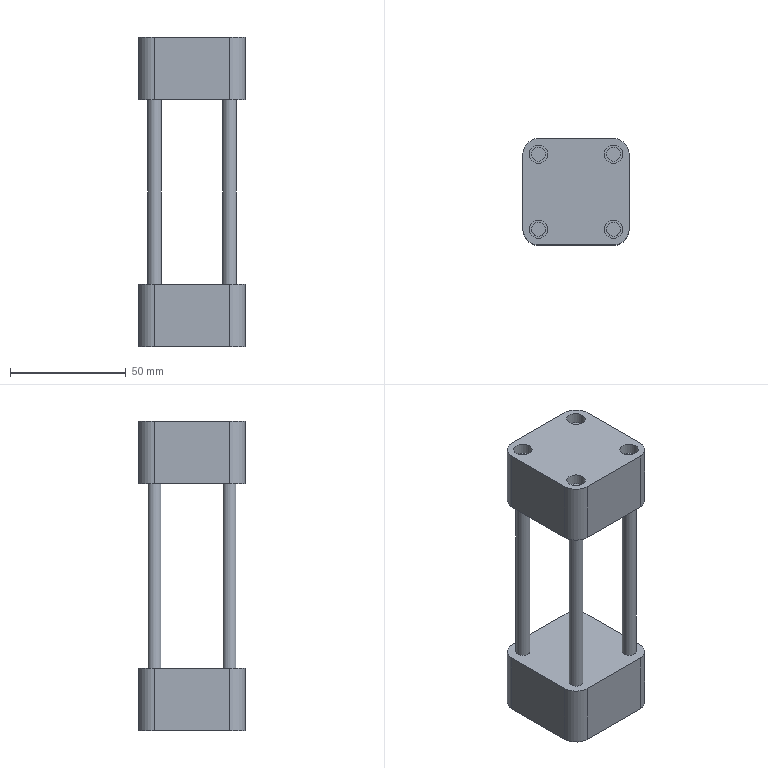Part | NX | features solid 2 | 1 solid | 48 faces | box 46 x 46 x 134 mm | volume 118030 mm3 | plane 24 | cylinder 24 | commonest cylinder face diameters 6 x8 13.5 x8 8 x4 6.667 x2 10 x2
STEP:
#1=CARTESIAN_POINT('',(312.,-98.75,-137.));
#2=VERTEX_POINT('',#1);
#3=CARTESIAN_POINT('',(312.,-131.25,-137.));
#4=VERTEX_POINT('',#3);
#5=CARTESIAN_POINT('',(312.,-92.,-137.));
#6=DIRECTION('',(0.,-1.,0.));
#7=VECTOR('',#6,1000.);
#8=LINE('',#5,#7);
#9=EDGE_CURVE('',#2,#4,#8,.T.);
#10=ORIENTED_EDGE('',*,*,#9,.F.);
#11=CARTESIAN_POINT('',(312.,-98.75,-164.));
#12=VERTEX_POINT('',#11);
#13=CARTESIAN_POINT('',(312.,-98.75,-164.));
#14=DIRECTION('',(0.,0.,-1.));
#15=VECTOR('',#14,1000.);
#16=LINE('',#13,#15);
#17=EDGE_CURVE('',#2,#12,#16,.T.);
#18=ORIENTED_EDGE('',*,*,#17,.T.);
#19=CARTESIAN_POINT('',(312.,-131.25,-164.));
#20=VERTEX_POINT('',#19);
#21=CARTESIAN_POINT('',(312.,-92.,-164.));
#22=DIRECTION('',(0.,-1.,0.));
#23=VECTOR('',#22,1000.);
#24=LINE('',#21,#23);
#25=EDGE_CURVE('',#12,#20,#24,.T.);
#26=ORIENTED_EDGE('',*,*,#25,.T.);
#27=CARTESIAN_POINT('',(312.,-131.25,-137.));
#28=DIRECTION('',(0.,0.,-1.));
#29=VECTOR('',#28,1000.);
#30=LINE('',#27,#29);
#31=EDGE_CURVE('',#20,#4,#30,.F.);
#32=ORIENTED_EDGE('',*,*,#31,.T.);
#33=EDGE_LOOP('',(#10,#18,#26,#32));
#34=FACE_BOUND('',#33,.T.);
#35=CARTESIAN_POINT('',(312.,-92.,-137.));
#36=DIRECTION('',(1.,0.,0.));
#37=DIRECTION('',(0.,1.,0.));
#38=AXIS2_PLACEMENT_3D('',#35,#36,#37);
#39=PLANE('',#38);
#40=ADVANCED_FACE('',(#34),#39,.F.);
#41=CARTESIAN_POINT('',(351.25,-138.,-137.));
#42=VERTEX_POINT('',#41);
#43=CARTESIAN_POINT('',(318.75,-138.,-137.));
#44=VERTEX_POINT('',#43);
#45=CARTESIAN_POINT('',(358.,-138.,-137.));
#46=DIRECTION('',(-1.,0.,0.));
#47=VECTOR('',#46,1000.);
#48=LINE('',#45,#47);
#49=EDGE_CURVE('',#42,#44,#48,.T.);
#50=ORIENTED_EDGE('',*,*,#49,.T.);
#51=CARTESIAN_POINT('',(318.75,-138.,-164.));
#52=VERTEX_POINT('',#51);
#53=CARTESIAN_POINT('',(318.75,-138.,-164.));
#54=DIRECTION('',(0.,0.,-1.));
#55=VECTOR('',#54,1000.);
#56=LINE('',#53,#55);
#57=EDGE_CURVE('',#44,#52,#56,.T.);
#58=ORIENTED_EDGE('',*,*,#57,.T.);
#59=CARTESIAN_POINT('',(351.25,-138.,-164.));
#60=VERTEX_POINT('',#59);
#61=CARTESIAN_POINT('',(358.,-138.,-164.));
#62=DIRECTION('',(-1.,0.,0.));
#63=VECTOR('',#62,1000.);
#64=LINE('',#61,#63);
#65=EDGE_CURVE('',#60,#52,#64,.T.);
#66=ORIENTED_EDGE('',*,*,#65,.F.);
#67=CARTESIAN_POINT('',(351.25,-138.,-137.));
#68=DIRECTION('',(0.,0.,-1.));
#69=VECTOR('',#68,1000.);
#70=LINE('',#67,#69);
#71=EDGE_CURVE('',#60,#42,#70,.F.);
#72=ORIENTED_EDGE('',*,*,#71,.T.);
#73=EDGE_LOOP('',(#50,#58,#66,#72));
#74=FACE_BOUND('',#73,.T.);
#75=CARTESIAN_POINT('',(358.,-138.,-137.));
#76=DIRECTION('',(0.,-1.,0.));
#77=DIRECTION('',(1.,0.,0.));
#78=AXIS2_PLACEMENT_3D('',#75,#76,#77);
#79=PLANE('',#78);
#80=ADVANCED_FACE('',(#74),#79,.T.);
#81=CARTESIAN_POINT('',(358.,-131.25,-164.));
#82=VERTEX_POINT('',#81);
#83=CARTESIAN_POINT('',(358.,-98.75,-164.));
#84=VERTEX_POINT('',#83);
#85=CARTESIAN_POINT('',(358.,-138.,-164.));
#86=DIRECTION('',(0.,1.,0.));
#87=VECTOR('',#86,1000.);
#88=LINE('',#85,#87);
#89=EDGE_CURVE('',#82,#84,#88,.T.);
#90=ORIENTED_EDGE('',*,*,#89,.T.);
#91=CARTESIAN_POINT('',(358.,-98.75,-137.));
#92=VERTEX_POINT('',#91);
#93=CARTESIAN_POINT('',(358.,-98.75,-137.));
#94=DIRECTION('',(0.,0.,-1.));
#95=VECTOR('',#94,1000.);
#96=LINE('',#93,#95);
#97=EDGE_CURVE('',#84,#92,#96,.F.);
#98=ORIENTED_EDGE('',*,*,#97,.T.);
#99=CARTESIAN_POINT('',(358.,-131.25,-137.));
#100=VERTEX_POINT('',#99);
#101=CARTESIAN_POINT('',(358.,-138.,-137.));
#102=DIRECTION('',(0.,1.,0.));
#103=VECTOR('',#102,1000.);
#104=LINE('',#101,#103);
#105=EDGE_CURVE('',#100,#92,#104,.T.);
#106=ORIENTED_EDGE('',*,*,#105,.F.);
#107=CARTESIAN_POINT('',(358.,-131.25,-164.));
#108=DIRECTION('',(0.,0.,-1.));
#109=VECTOR('',#108,1000.);
#110=LINE('',#107,#109);
#111=EDGE_CURVE('',#100,#82,#110,.T.);
#112=ORIENTED_EDGE('',*,*,#111,.T.);
#113=EDGE_LOOP('',(#90,#98,#106,#112));
#114=FACE_BOUND('',#113,.T.);
#115=CARTESIAN_POINT('',(358.,-138.,-137.));
#116=DIRECTION('',(-1.,0.,0.));
#117=DIRECTION('',(0.,-1.,0.));
#118=AXIS2_PLACEMENT_3D('',#115,#116,#117);
#119=PLANE('',#118);
#120=ADVANCED_FACE('',(#114),#119,.F.);
#121=CARTESIAN_POINT('',(341.5,-92.,-151.833));
#122=VERTEX_POINT('',#121);
#123=CARTESIAN_POINT('',(341.5,-92.,-148.5));
#124=DIRECTION('',(0.,-1.,0.));
#125=DIRECTION('',(0.,0.,-1.));
#126=AXIS2_PLACEMENT_3D('',#123,#124,#125);
#127=CIRCLE('',#126,3.333);
#128=EDGE_CURVE('',#122,#122,#127,.T.);
#129=ORIENTED_EDGE('',*,*,#128,.T.);
#130=EDGE_LOOP('',(#129));
#131=FACE_BOUND('',#130,.T.);
#132=CARTESIAN_POINT('',(331.,-92.,-156.));
#133=VERTEX_POINT('',#132);
#134=CARTESIAN_POINT('',(331.,-92.,-151.));
#135=DIRECTION('',(0.,-1.,0.));
#136=DIRECTION('',(0.,0.,-1.));
#137=AXIS2_PLACEMENT_3D('',#134,#135,#136);
#138=CIRCLE('',#137,5.);
#139=EDGE_CURVE('',#133,#133,#138,.T.);
#140=ORIENTED_EDGE('',*,*,#139,.T.);
#141=EDGE_LOOP('',(#140));
#142=FACE_BOUND('',#141,.T.);
#143=CARTESIAN_POINT('',(318.75,-92.,-164.));
#144=VERTEX_POINT('',#143);
#145=CARTESIAN_POINT('',(351.25,-92.,-164.));
#146=VERTEX_POINT('',#145);
#147=CARTESIAN_POINT('',(312.,-92.,-164.));
#148=DIRECTION('',(1.,0.,0.));
#149=VECTOR('',#148,1000.);
#150=LINE('',#147,#149);
#151=EDGE_CURVE('',#144,#146,#150,.T.);
#152=ORIENTED_EDGE('',*,*,#151,.F.);
#153=CARTESIAN_POINT('',(318.75,-92.,-137.));
#154=VERTEX_POINT('',#153);
#155=CARTESIAN_POINT('',(318.75,-92.,-137.));
#156=DIRECTION('',(0.,0.,-1.));
#157=VECTOR('',#156,1000.);
#158=LINE('',#155,#157);
#159=EDGE_CURVE('',#144,#154,#158,.F.);
#160=ORIENTED_EDGE('',*,*,#159,.T.);
#161=CARTESIAN_POINT('',(351.25,-92.,-137.));
#162=VERTEX_POINT('',#161);
#163=CARTESIAN_POINT('',(312.,-92.,-137.));
#164=DIRECTION('',(1.,0.,0.));
#165=VECTOR('',#164,1000.);
#166=LINE('',#163,#165);
#167=EDGE_CURVE('',#154,#162,#166,.T.);
#168=ORIENTED_EDGE('',*,*,#167,.T.);
#169=CARTESIAN_POINT('',(351.25,-92.,-164.));
#170=DIRECTION('',(0.,0.,-1.));
#171=VECTOR('',#170,1000.);
#172=LINE('',#169,#171);
#173=EDGE_CURVE('',#162,#146,#172,.T.);
#174=ORIENTED_EDGE('',*,*,#173,.T.);
#175=EDGE_LOOP('',(#152,#160,#168,#174));
#176=FACE_BOUND('',#175,.T.);
#177=CARTESIAN_POINT('',(312.,-92.,-137.));
#178=DIRECTION('',(0.,1.,0.));
#179=DIRECTION('',(0.,0.,1.));
#180=AXIS2_PLACEMENT_3D('',#177,#178,#179);
#181=PLANE('',#180);
#182=ADVANCED_FACE('',(#131,#142,#176),#181,.T.);
#183=CARTESIAN_POINT('',(348.25,-98.75,-137.));
#184=VERTEX_POINT('',#183);
#185=CARTESIAN_POINT('',(351.25,-98.75,-137.));
#186=DIRECTION('',(0.,0.,1.));
#187=DIRECTION('',(-1.,0.,0.));
#188=AXIS2_PLACEMENT_3D('',#185,#186,#187);
#189=CIRCLE('',#188,3.);
#190=EDGE_CURVE('',#184,#184,#189,.T.);
#191=ORIENTED_EDGE('',*,*,#190,.F.);
#192=EDGE_LOOP('',(#191));
#193=FACE_BOUND('',#192,.T.);
#194=CARTESIAN_POINT('',(321.75,-98.75,-137.));
#195=VERTEX_POINT('',#194);
#196=CARTESIAN_POINT('',(318.75,-98.75,-137.));
#197=DIRECTION('',(0.,0.,-1.));
#198=DIRECTION('',(1.,0.,0.));
#199=AXIS2_PLACEMENT_3D('',#196,#197,#198);
#200=CIRCLE('',#199,3.);
#201=EDGE_CURVE('',#195,#195,#200,.T.);
#202=ORIENTED_EDGE('',*,*,#201,.T.);
#203=EDGE_LOOP('',(#202));
#204=FACE_BOUND('',#203,.T.);
#205=CARTESIAN_POINT('',(348.25,-131.25,-137.));
#206=VERTEX_POINT('',#205);
#207=CARTESIAN_POINT('',(351.25,-131.25,-137.));
#208=DIRECTION('',(0.,0.,-1.));
#209=DIRECTION('',(-1.,0.,0.));
#210=AXIS2_PLACEMENT_3D('',#207,#208,#209);
#211=CIRCLE('',#210,3.);
#212=EDGE_CURVE('',#206,#206,#211,.T.);
#213=ORIENTED_EDGE('',*,*,#212,.T.);
#214=EDGE_LOOP('',(#213));
#215=FACE_BOUND('',#214,.T.);
#216=CARTESIAN_POINT('',(321.75,-131.25,-137.));
#217=VERTEX_POINT('',#216);
#218=CARTESIAN_POINT('',(318.75,-131.25,-137.));
#219=DIRECTION('',(0.,0.,1.));
#220=DIRECTION('',(1.,0.,0.));
#221=AXIS2_PLACEMENT_3D('',#218,#219,#220);
#222=CIRCLE('',#221,3.);
#223=EDGE_CURVE('',#217,#217,#222,.T.);
#224=ORIENTED_EDGE('',*,*,#223,.F.);
#225=EDGE_LOOP('',(#224));
#226=FACE_BOUND('',#225,.T.);
#227=ORIENTED_EDGE('',*,*,#167,.F.);
#228=CARTESIAN_POINT('',(318.75,-98.75,-137.));
#229=DIRECTION('',(0.,0.,-1.));
#230=DIRECTION('',(-1.,0.,0.));
#231=AXIS2_PLACEMENT_3D('',#228,#229,#230);
#232=CIRCLE('',#231,6.75);
#233=EDGE_CURVE('',#154,#2,#232,.F.);
#234=ORIENTED_EDGE('',*,*,#233,.T.);
#235=ORIENTED_EDGE('',*,*,#9,.T.);
#236=CARTESIAN_POINT('',(318.75,-131.25,-137.));
#237=DIRECTION('',(0.,0.,-1.));
#238=DIRECTION('',(-1.,0.,0.));
#239=AXIS2_PLACEMENT_3D('',#236,#237,#238);
#240=CIRCLE('',#239,6.75);
#241=EDGE_CURVE('',#4,#44,#240,.F.);
#242=ORIENTED_EDGE('',*,*,#241,.T.);
#243=ORIENTED_EDGE('',*,*,#49,.F.);
#244=CARTESIAN_POINT('',(351.25,-131.25,-137.));
#245=DIRECTION('',(0.,0.,-1.));
#246=DIRECTION('',(-1.,0.,0.));
#247=AXIS2_PLACEMENT_3D('',#244,#245,#246);
#248=CIRCLE('',#247,6.75);
#249=EDGE_CURVE('',#42,#100,#248,.F.);
#250=ORIENTED_EDGE('',*,*,#249,.T.);
#251=ORIENTED_EDGE('',*,*,#105,.T.);
#252=CARTESIAN_POINT('',(351.25,-98.75,-137.));
#253=DIRECTION('',(0.,0.,-1.));
#254=DIRECTION('',(-1.,0.,0.));
#255=AXIS2_PLACEMENT_3D('',#252,#253,#254);
#256=CIRCLE('',#255,6.75);
#257=EDGE_CURVE('',#92,#162,#256,.F.);
#258=ORIENTED_EDGE('',*,*,#257,.T.);
#259=EDGE_LOOP('',(#227,#234,#235,#242,#243,#250,#251,#258));
#260=FACE_BOUND('',#259,.T.);
#261=CARTESIAN_POINT('',(312.,-138.,-137.));
#262=DIRECTION('',(0.,0.,-1.));
#263=DIRECTION('',(-1.,0.,0.));
#264=AXIS2_PLACEMENT_3D('',#261,#262,#263);
#265=PLANE('',#264);
#266=ADVANCED_FACE('',(#193,#204,#215,#226,#260),#265,.F.);
#267=ORIENTED_EDGE('',*,*,#25,.F.);
#268=CARTESIAN_POINT('',(318.75,-98.75,-164.));
#269=DIRECTION('',(0.,0.,-1.));
#270=DIRECTION('',(-1.,0.,0.));
#271=AXIS2_PLACEMENT_3D('',#268,#269,#270);
#272=CIRCLE('',#271,6.75);
#273=EDGE_CURVE('',#12,#144,#272,.T.);
#274=ORIENTED_EDGE('',*,*,#273,.T.);
#275=ORIENTED_EDGE('',*,*,#151,.T.);
#276=CARTESIAN_POINT('',(351.25,-98.75,-164.));
#277=DIRECTION('',(0.,0.,-1.));
#278=DIRECTION('',(-1.,0.,0.));
#279=AXIS2_PLACEMENT_3D('',#276,#277,#278);
#280=CIRCLE('',#279,6.75);
#281=EDGE_CURVE('',#146,#84,#280,.T.);
#282=ORIENTED_EDGE('',*,*,#281,.T.);
#283=ORIENTED_EDGE('',*,*,#89,.F.);
#284=CARTESIAN_POINT('',(351.25,-131.25,-164.));
#285=DIRECTION('',(0.,0.,-1.));
#286=DIRECTION('',(-1.,0.,0.));
#287=AXIS2_PLACEMENT_3D('',#284,#285,#286);
#288=CIRCLE('',#287,6.75);
#289=EDGE_CURVE('',#82,#60,#288,.T.);
#290=ORIENTED_EDGE('',*,*,#289,.T.);
#291=ORIENTED_EDGE('',*,*,#65,.T.);
#292=CARTESIAN_POINT('',(318.75,-131.25,-164.));
#293=DIRECTION('',(0.,0.,-1.));
#294=DIRECTION('',(-1.,0.,0.));
#295=AXIS2_PLACEMENT_3D('',#292,#293,#294);
#296=CIRCLE('',#295,6.75);
#297=EDGE_CURVE('',#52,#20,#296,.T.);
#298=ORIENTED_EDGE('',*,*,#297,.T.);
#299=EDGE_LOOP('',(#267,#274,#275,#282,#283,#290,#291,#298));
#300=FACE_BOUND('',#299,.T.);
#301=CARTESIAN_POINT('',(312.,-138.,-164.));
#302=DIRECTION('',(0.,0.,-1.));
#303=DIRECTION('',(-1.,0.,0.));
#304=AXIS2_PLACEMENT_3D('',#301,#302,#303);
#305=PLANE('',#304);
#306=ADVANCED_FACE('',(#300),#305,.T.);
#307=ORIENTED_EDGE('',*,*,#233,.F.);
#308=ORIENTED_EDGE('',*,*,#159,.F.);
#309=ORIENTED_EDGE('',*,*,#273,.F.);
#310=ORIENTED_EDGE('',*,*,#17,.F.);
#311=EDGE_LOOP('',(#307,#308,#309,#310));
#312=FACE_BOUND('',#311,.T.);
#313=CARTESIAN_POINT('',(318.75,-98.75,-137.));
#314=DIRECTION('',(0.,0.,1.));
#315=DIRECTION('',(1.,0.,0.));
#316=AXIS2_PLACEMENT_3D('',#313,#314,#315);
#317=CYLINDRICAL_SURFACE('',#316,6.75);
#318=ADVANCED_FACE('',(#312),#317,.T.);
#319=ORIENTED_EDGE('',*,*,#241,.F.);
#320=ORIENTED_EDGE('',*,*,#31,.F.);
#321=ORIENTED_EDGE('',*,*,#297,.F.);
#322=ORIENTED_EDGE('',*,*,#57,.F.);
#323=EDGE_LOOP('',(#319,#320,#321,#322));
#324=FACE_BOUND('',#323,.T.);
#325=CARTESIAN_POINT('',(318.75,-131.25,-137.));
#326=DIRECTION('',(0.,0.,1.));
#327=DIRECTION('',(1.,0.,0.));
#328=AXIS2_PLACEMENT_3D('',#325,#326,#327);
#329=CYLINDRICAL_SURFACE('',#328,6.75);
#330=ADVANCED_FACE('',(#324),#329,.T.);
#331=ORIENTED_EDGE('',*,*,#257,.F.);
#332=ORIENTED_EDGE('',*,*,#97,.F.);
#333=ORIENTED_EDGE('',*,*,#281,.F.);
#334=ORIENTED_EDGE('',*,*,#173,.F.);
#335=EDGE_LOOP('',(#331,#332,#333,#334));
#336=FACE_BOUND('',#335,.T.);
#337=CARTESIAN_POINT('',(351.25,-98.75,-137.));
#338=DIRECTION('',(0.,0.,1.));
#339=DIRECTION('',(1.,0.,0.));
#340=AXIS2_PLACEMENT_3D('',#337,#338,#339);
#341=CYLINDRICAL_SURFACE('',#340,6.75);
#342=ADVANCED_FACE('',(#336),#341,.T.);
#343=ORIENTED_EDGE('',*,*,#249,.F.);
#344=ORIENTED_EDGE('',*,*,#71,.F.);
#345=ORIENTED_EDGE('',*,*,#289,.F.);
#346=ORIENTED_EDGE('',*,*,#111,.F.);
#347=EDGE_LOOP('',(#343,#344,#345,#346));
#348=FACE_BOUND('',#347,.T.);
#349=CARTESIAN_POINT('',(351.25,-131.25,-137.));
#350=DIRECTION('',(0.,0.,1.));
#351=DIRECTION('',(1.,0.,0.));
#352=AXIS2_PLACEMENT_3D('',#349,#350,#351);
#353=CYLINDRICAL_SURFACE('',#352,6.75);
#354=ADVANCED_FACE('',(#348),#353,.T.);
#355=CARTESIAN_POINT('',(315.75,-131.25,-57.));
#356=VERTEX_POINT('',#355);
#357=CARTESIAN_POINT('',(318.75,-131.25,-57.));
#358=DIRECTION('',(0.,0.,-1.));
#359=DIRECTION('',(-1.,0.,0.));
#360=AXIS2_PLACEMENT_3D('',#357,#358,#359);
#361=CIRCLE('',#360,3.);
#362=EDGE_CURVE('',#356,#356,#361,.F.);
#363=ORIENTED_EDGE('',*,*,#362,.F.);
#364=EDGE_LOOP('',(#363));
#365=FACE_BOUND('',#364,.T.);
#366=ORIENTED_EDGE('',*,*,#223,.T.);
#367=EDGE_LOOP('',(#366));
#368=FACE_BOUND('',#367,.T.);
#369=CARTESIAN_POINT('',(318.75,-131.25,-137.));
#370=DIRECTION('',(0.,0.,1.));
#371=DIRECTION('',(1.,0.,0.));
#372=AXIS2_PLACEMENT_3D('',#369,#370,#371);
#373=CYLINDRICAL_SURFACE('',#372,3.);
#374=ADVANCED_FACE('',(#365,#368),#373,.T.);
#375=CARTESIAN_POINT('',(348.25,-131.25,-57.));
#376=VERTEX_POINT('',#375);
#377=CARTESIAN_POINT('',(351.25,-131.25,-57.));
#378=DIRECTION('',(0.,0.,-1.));
#379=DIRECTION('',(-1.,0.,0.));
#380=AXIS2_PLACEMENT_3D('',#377,#378,#379);
#381=CIRCLE('',#380,3.);
#382=EDGE_CURVE('',#376,#376,#381,.F.);
#383=ORIENTED_EDGE('',*,*,#382,.F.);
#384=EDGE_LOOP('',(#383));
#385=FACE_BOUND('',#384,.T.);
#386=ORIENTED_EDGE('',*,*,#212,.F.);
#387=EDGE_LOOP('',(#386));
#388=FACE_BOUND('',#387,.T.);
#389=CARTESIAN_POINT('',(351.25,-131.25,-137.));
#390=DIRECTION('',(0.,0.,1.));
#391=DIRECTION('',(-1.,0.,0.));
#392=AXIS2_PLACEMENT_3D('',#389,#390,#391);
#393=CYLINDRICAL_SURFACE('',#392,3.);
#394=ADVANCED_FACE('',(#385,#388),#393,.T.);
#395=CARTESIAN_POINT('',(315.75,-98.75,-57.));
#396=VERTEX_POINT('',#395);
#397=CARTESIAN_POINT('',(318.75,-98.75,-57.));
#398=DIRECTION('',(0.,0.,-1.));
#399=DIRECTION('',(-1.,0.,0.));
#400=AXIS2_PLACEMENT_3D('',#397,#398,#399);
#401=CIRCLE('',#400,3.);
#402=EDGE_CURVE('',#396,#396,#401,.F.);
#403=ORIENTED_EDGE('',*,*,#402,.F.);
#404=EDGE_LOOP('',(#403));
#405=FACE_BOUND('',#404,.T.);
#406=ORIENTED_EDGE('',*,*,#201,.F.);
#407=EDGE_LOOP('',(#406));
#408=FACE_BOUND('',#407,.T.);
#409=CARTESIAN_POINT('',(318.75,-98.75,-137.));
#410=DIRECTION('',(0.,0.,1.));
#411=DIRECTION('',(1.,0.,0.));
#412=AXIS2_PLACEMENT_3D('',#409,#410,#411);
#413=CYLINDRICAL_SURFACE('',#412,3.);
#414=ADVANCED_FACE('',(#405,#408),#413,.T.);
#415=CARTESIAN_POINT('',(348.25,-98.75,-57.));
#416=VERTEX_POINT('',#415);
#417=CARTESIAN_POINT('',(351.25,-98.75,-57.));
#418=DIRECTION('',(0.,0.,-1.));
#419=DIRECTION('',(-1.,0.,0.));
#420=AXIS2_PLACEMENT_3D('',#417,#418,#419);
#421=CIRCLE('',#420,3.);
#422=EDGE_CURVE('',#416,#416,#421,.F.);
#423=ORIENTED_EDGE('',*,*,#422,.F.);
#424=EDGE_LOOP('',(#423));
#425=FACE_BOUND('',#424,.T.);
#426=ORIENTED_EDGE('',*,*,#190,.T.);
#427=EDGE_LOOP('',(#426));
#428=FACE_BOUND('',#427,.T.);
#429=CARTESIAN_POINT('',(351.25,-98.75,-137.));
#430=DIRECTION('',(0.,0.,1.));
#431=DIRECTION('',(-1.,0.,0.));
#432=AXIS2_PLACEMENT_3D('',#429,#430,#431);
#433=CYLINDRICAL_SURFACE('',#432,3.);
#434=ADVANCED_FACE('',(#425,#428),#433,.T.);
#435=CARTESIAN_POINT('',(331.,-97.,-156.));
#436=VERTEX_POINT('',#435);
#437=CARTESIAN_POINT('',(331.,-97.,-151.));
#438=DIRECTION('',(0.,-1.,0.));
#439=DIRECTION('',(0.,0.,-1.));
#440=AXIS2_PLACEMENT_3D('',#437,#438,#439);
#441=CIRCLE('',#440,5.);
#442=EDGE_CURVE('',#436,#436,#441,.T.);
#443=ORIENTED_EDGE('',*,*,#442,.F.);
#444=EDGE_LOOP('',(#443));
#445=FACE_BOUND('',#444,.T.);
#446=CARTESIAN_POINT('',(331.,-97.,-151.));
#447=DIRECTION('',(0.,-1.,0.));
#448=DIRECTION('',(0.,0.,-1.));
#449=AXIS2_PLACEMENT_3D('',#446,#447,#448);
#450=PLANE('',#449);
#451=ADVANCED_FACE('',(#445),#450,.F.);
#452=ORIENTED_EDGE('',*,*,#442,.T.);
#453=EDGE_LOOP('',(#452));
#454=FACE_BOUND('',#453,.T.);
#455=ORIENTED_EDGE('',*,*,#139,.F.);
#456=EDGE_LOOP('',(#455));
#457=FACE_BOUND('',#456,.T.);
#458=CARTESIAN_POINT('',(331.,-92.,-151.));
#459=DIRECTION('',(0.,-1.,0.));
#460=DIRECTION('',(0.,0.,-1.));
#461=AXIS2_PLACEMENT_3D('',#458,#459,#460);
#462=CYLINDRICAL_SURFACE('',#461,5.);
#463=ADVANCED_FACE('',(#454,#457),#462,.F.);
#464=CARTESIAN_POINT('',(341.5,-97.,-151.833));
#465=VERTEX_POINT('',#464);
#466=CARTESIAN_POINT('',(341.5,-97.,-148.5));
#467=DIRECTION('',(0.,-1.,0.));
#468=DIRECTION('',(0.,0.,-1.));
#469=AXIS2_PLACEMENT_3D('',#466,#467,#468);
#470=CIRCLE('',#469,3.333);
#471=EDGE_CURVE('',#465,#465,#470,.T.);
#472=ORIENTED_EDGE('',*,*,#471,.F.);
#473=EDGE_LOOP('',(#472));
#474=FACE_BOUND('',#473,.T.);
#475=CARTESIAN_POINT('',(341.5,-97.,-148.5));
#476=DIRECTION('',(0.,-1.,0.));
#477=DIRECTION('',(0.,0.,-1.));
#478=AXIS2_PLACEMENT_3D('',#475,#476,#477);
#479=PLANE('',#478);
#480=ADVANCED_FACE('',(#474),#479,.F.);
#481=ORIENTED_EDGE('',*,*,#471,.T.);
#482=EDGE_LOOP('',(#481));
#483=FACE_BOUND('',#482,.T.);
#484=ORIENTED_EDGE('',*,*,#128,.F.);
#485=EDGE_LOOP('',(#484));
#486=FACE_BOUND('',#485,.T.);
#487=CARTESIAN_POINT('',(341.5,-92.,-148.5));
#488=DIRECTION('',(0.,-1.,0.));
#489=DIRECTION('',(0.,0.,-1.));
#490=AXIS2_PLACEMENT_3D('',#487,#488,#489);
#491=CYLINDRICAL_SURFACE('',#490,3.333);
#492=ADVANCED_FACE('',(#483,#486),#491,.F.);
#493=CARTESIAN_POINT('',(358.,-131.25,-57.));
#494=VERTEX_POINT('',#493);
#495=CARTESIAN_POINT('',(358.,-98.75,-57.));
#496=VERTEX_POINT('',#495);
#497=CARTESIAN_POINT('',(358.,-138.,-57.));
#498=DIRECTION('',(0.,1.,0.));
#499=VECTOR('',#498,1000.);
#500=LINE('',#497,#499);
#501=EDGE_CURVE('',#494,#496,#500,.T.);
#502=ORIENTED_EDGE('',*,*,#501,.T.);
#503=CARTESIAN_POINT('',(358.,-98.75,-30.));
#504=VERTEX_POINT('',#503);
#505=CARTESIAN_POINT('',(358.,-98.75,-30.));
#506=DIRECTION('',(0.,0.,1.));
#507=VECTOR('',#506,1000.);
#508=LINE('',#505,#507);
#509=EDGE_CURVE('',#496,#504,#508,.T.);
#510=ORIENTED_EDGE('',*,*,#509,.T.);
#511=CARTESIAN_POINT('',(358.,-131.25,-30.));
#512=VERTEX_POINT('',#511);
#513=CARTESIAN_POINT('',(358.,-138.,-30.));
#514=DIRECTION('',(0.,1.,0.));
#515=VECTOR('',#514,1000.);
#516=LINE('',#513,#515);
#517=EDGE_CURVE('',#512,#504,#516,.T.);
#518=ORIENTED_EDGE('',*,*,#517,.F.);
#519=CARTESIAN_POINT('',(358.,-131.25,-57.));
#520=DIRECTION('',(0.,0.,1.));
#521=VECTOR('',#520,1000.);
#522=LINE('',#519,#521);
#523=EDGE_CURVE('',#512,#494,#522,.F.);
#524=ORIENTED_EDGE('',*,*,#523,.T.);
#525=EDGE_LOOP('',(#502,#510,#518,#524));
#526=FACE_BOUND('',#525,.T.);
#527=CARTESIAN_POINT('',(358.,-138.,-57.));
#528=DIRECTION('',(1.,0.,0.));
#529=DIRECTION('',(0.,1.,0.));
#530=AXIS2_PLACEMENT_3D('',#527,#528,#529);
#531=PLANE('',#530);
#532=ADVANCED_FACE('',(#526),#531,.T.);
#533=CARTESIAN_POINT('',(341.5,-92.,-48.833));
#534=VERTEX_POINT('',#533);
#535=CARTESIAN_POINT('',(341.5,-92.,-45.5));
#536=DIRECTION('',(0.,-1.,0.));
#537=DIRECTION('',(0.,0.,-1.));
#538=AXIS2_PLACEMENT_3D('',#535,#536,#537);
#539=CIRCLE('',#538,3.333);
#540=EDGE_CURVE('',#534,#534,#539,.T.);
#541=ORIENTED_EDGE('',*,*,#540,.T.);
#542=EDGE_LOOP('',(#541));
#543=FACE_BOUND('',#542,.T.);
#544=CARTESIAN_POINT('',(331.,-92.,-48.));
#545=VERTEX_POINT('',#544);
#546=CARTESIAN_POINT('',(331.,-92.,-43.));
#547=DIRECTION('',(0.,-1.,0.));
#548=DIRECTION('',(0.,0.,-1.));
#549=AXIS2_PLACEMENT_3D('',#546,#547,#548);
#550=CIRCLE('',#549,5.);
#551=EDGE_CURVE('',#545,#545,#550,.T.);
#552=ORIENTED_EDGE('',*,*,#551,.T.);
#553=EDGE_LOOP('',(#552));
#554=FACE_BOUND('',#553,.T.);
#555=CARTESIAN_POINT('',(318.75,-92.,-30.));
#556=VERTEX_POINT('',#555);
#557=CARTESIAN_POINT('',(351.25,-92.,-30.));
#558=VERTEX_POINT('',#557);
#559=CARTESIAN_POINT('',(312.,-92.,-30.));
#560=DIRECTION('',(1.,0.,0.));
#561=VECTOR('',#560,1000.);
#562=LINE('',#559,#561);
#563=EDGE_CURVE('',#556,#558,#562,.T.);
#564=ORIENTED_EDGE('',*,*,#563,.T.);
#565=CARTESIAN_POINT('',(351.25,-92.,-57.));
#566=VERTEX_POINT('',#565);
#567=CARTESIAN_POINT('',(351.25,-92.,-57.));
#568=DIRECTION('',(0.,0.,1.));
#569=VECTOR('',#568,1000.);
#570=LINE('',#567,#569);
#571=EDGE_CURVE('',#558,#566,#570,.F.);
#572=ORIENTED_EDGE('',*,*,#571,.T.);
#573=CARTESIAN_POINT('',(318.75,-92.,-57.));
#574=VERTEX_POINT('',#573);
#575=CARTESIAN_POINT('',(312.,-92.,-57.));
#576=DIRECTION('',(1.,0.,0.));
#577=VECTOR('',#576,1000.);
#578=LINE('',#575,#577);
#579=EDGE_CURVE('',#574,#566,#578,.T.);
#580=ORIENTED_EDGE('',*,*,#579,.F.);
#581=CARTESIAN_POINT('',(318.75,-92.,-30.));
#582=DIRECTION('',(0.,0.,1.));
#583=VECTOR('',#582,1000.);
#584=LINE('',#581,#583);
#585=EDGE_CURVE('',#574,#556,#584,.T.);
#586=ORIENTED_EDGE('',*,*,#585,.T.);
#587=EDGE_LOOP('',(#564,#572,#580,#586));
#588=FACE_BOUND('',#587,.T.);
#589=CARTESIAN_POINT('',(312.,-92.,-57.));
#590=DIRECTION('',(0.,-1.,0.));
#591=DIRECTION('',(0.,0.,-1.));
#592=AXIS2_PLACEMENT_3D('',#589,#590,#591);
#593=PLANE('',#592);
#594=ADVANCED_FACE('',(#543,#554,#588),#593,.F.);
#595=CARTESIAN_POINT('',(312.,-98.75,-57.));
#596=VERTEX_POINT('',#595);
#597=CARTESIAN_POINT('',(312.,-131.25,-57.));
#598=VERTEX_POINT('',#597);
#599=CARTESIAN_POINT('',(312.,-92.,-57.));
#600=DIRECTION('',(0.,-1.,0.));
#601=VECTOR('',#600,1000.);
#602=LINE('',#599,#601);
#603=EDGE_CURVE('',#596,#598,#602,.T.);
#604=ORIENTED_EDGE('',*,*,#603,.T.);
#605=CARTESIAN_POINT('',(312.,-131.25,-30.));
#606=VERTEX_POINT('',#605);
#607=CARTESIAN_POINT('',(312.,-131.25,-30.));
#608=DIRECTION('',(0.,0.,1.));
#609=VECTOR('',#608,1000.);
#610=LINE('',#607,#609);
#611=EDGE_CURVE('',#598,#606,#610,.T.);
#612=ORIENTED_EDGE('',*,*,#611,.T.);
#613=CARTESIAN_POINT('',(312.,-98.75,-30.));
#614=VERTEX_POINT('',#613);
#615=CARTESIAN_POINT('',(312.,-92.,-30.));
#616=DIRECTION('',(0.,-1.,0.));
#617=VECTOR('',#616,1000.);
#618=LINE('',#615,#617);
#619=EDGE_CURVE('',#614,#606,#618,.T.);
#620=ORIENTED_EDGE('',*,*,#619,.F.);
#621=CARTESIAN_POINT('',(312.,-98.75,-57.));
#622=DIRECTION('',(0.,0.,1.));
#623=VECTOR('',#622,1000.);
#624=LINE('',#621,#623);
#625=EDGE_CURVE('',#614,#596,#624,.F.);
#626=ORIENTED_EDGE('',*,*,#625,.T.);
#627=EDGE_LOOP('',(#604,#612,#620,#626));
#628=FACE_BOUND('',#627,.T.);
#629=CARTESIAN_POINT('',(312.,-92.,-57.));
#630=DIRECTION('',(-1.,0.,0.));
#631=DIRECTION('',(0.,-1.,0.));
#632=AXIS2_PLACEMENT_3D('',#629,#630,#631);
#633=PLANE('',#632);
#634=ADVANCED_FACE('',(#628),#633,.T.);
#635=CARTESIAN_POINT('',(351.25,-138.,-57.));
#636=VERTEX_POINT('',#635);
#637=CARTESIAN_POINT('',(318.75,-138.,-57.));
#638=VERTEX_POINT('',#637);
#639=CARTESIAN_POINT('',(358.,-138.,-57.));
#640=DIRECTION('',(-1.,0.,0.));
#641=VECTOR('',#640,1000.);
#642=LINE('',#639,#641);
#643=EDGE_CURVE('',#636,#638,#642,.T.);
#644=ORIENTED_EDGE('',*,*,#643,.F.);
#645=CARTESIAN_POINT('',(351.25,-138.,-30.));
#646=VERTEX_POINT('',#645);
#647=CARTESIAN_POINT('',(351.25,-138.,-30.));
#648=DIRECTION('',(0.,0.,1.));
#649=VECTOR('',#648,1000.);
#650=LINE('',#647,#649);
#651=EDGE_CURVE('',#636,#646,#650,.T.);
#652=ORIENTED_EDGE('',*,*,#651,.T.);
#653=CARTESIAN_POINT('',(318.75,-138.,-30.));
#654=VERTEX_POINT('',#653);
#655=CARTESIAN_POINT('',(358.,-138.,-30.));
#656=DIRECTION('',(-1.,0.,0.));
#657=VECTOR('',#656,1000.);
#658=LINE('',#655,#657);
#659=EDGE_CURVE('',#646,#654,#658,.T.);
#660=ORIENTED_EDGE('',*,*,#659,.T.);
#661=CARTESIAN_POINT('',(318.75,-138.,-57.));
#662=DIRECTION('',(0.,0.,1.));
#663=VECTOR('',#662,1000.);
#664=LINE('',#661,#663);
#665=EDGE_CURVE('',#654,#638,#664,.F.);
#666=ORIENTED_EDGE('',*,*,#665,.T.);
#667=EDGE_LOOP('',(#644,#652,#660,#666));
#668=FACE_BOUND('',#667,.T.);
#669=CARTESIAN_POINT('',(358.,-138.,-57.));
#670=DIRECTION('',(0.,1.,0.));
#671=DIRECTION('',(-1.,0.,0.));
#672=AXIS2_PLACEMENT_3D('',#669,#670,#671);
#673=PLANE('',#672);
#674=ADVANCED_FACE('',(#668),#673,.F.);
#675=ORIENTED_EDGE('',*,*,#362,.T.);
#676=EDGE_LOOP('',(#675));
#677=FACE_BOUND('',#676,.T.);
#678=ORIENTED_EDGE('',*,*,#382,.T.);
#679=EDGE_LOOP('',(#678));
#680=FACE_BOUND('',#679,.T.);
#681=ORIENTED_EDGE('',*,*,#402,.T.);
#682=EDGE_LOOP('',(#681));
#683=FACE_BOUND('',#682,.T.);
#684=ORIENTED_EDGE('',*,*,#422,.T.);
#685=EDGE_LOOP('',(#684));
#686=FACE_BOUND('',#685,.T.);
#687=ORIENTED_EDGE('',*,*,#579,.T.);
#688=CARTESIAN_POINT('',(351.25,-98.75,-57.));
#689=DIRECTION('',(0.,0.,-1.));
#690=DIRECTION('',(-1.,0.,0.));
#691=AXIS2_PLACEMENT_3D('',#688,#689,#690);
#692=CIRCLE('',#691,6.75);
#693=EDGE_CURVE('',#566,#496,#692,.T.);
#694=ORIENTED_EDGE('',*,*,#693,.T.);
#695=ORIENTED_EDGE('',*,*,#501,.F.);
#696=CARTESIAN_POINT('',(351.25,-131.25,-57.));
#697=DIRECTION('',(0.,0.,-1.));
#698=DIRECTION('',(-1.,0.,0.));
#699=AXIS2_PLACEMENT_3D('',#696,#697,#698);
#700=CIRCLE('',#699,6.75);
#701=EDGE_CURVE('',#494,#636,#700,.T.);
#702=ORIENTED_EDGE('',*,*,#701,.T.);
#703=ORIENTED_EDGE('',*,*,#643,.T.);
#704=CARTESIAN_POINT('',(318.75,-131.25,-57.));
#705=DIRECTION('',(0.,0.,-1.));
#706=DIRECTION('',(-1.,0.,0.));
#707=AXIS2_PLACEMENT_3D('',#704,#705,#706);
#708=CIRCLE('',#707,6.75);
#709=EDGE_CURVE('',#638,#598,#708,.T.);
#710=ORIENTED_EDGE('',*,*,#709,.T.);
#711=ORIENTED_EDGE('',*,*,#603,.F.);
#712=CARTESIAN_POINT('',(318.75,-98.75,-57.));
#713=DIRECTION('',(0.,0.,-1.));
#714=DIRECTION('',(-1.,0.,0.));
#715=AXIS2_PLACEMENT_3D('',#712,#713,#714);
#716=CIRCLE('',#715,6.75);
#717=EDGE_CURVE('',#596,#574,#716,.T.);
#718=ORIENTED_EDGE('',*,*,#717,.T.);
#719=EDGE_LOOP('',(#687,#694,#695,#702,#703,#710,#711,#718));
#720=FACE_BOUND('',#719,.T.);
#721=CARTESIAN_POINT('',(358.,-92.,-57.));
#722=DIRECTION('',(0.,0.,-1.));
#723=DIRECTION('',(-1.,0.,0.));
#724=AXIS2_PLACEMENT_3D('',#721,#722,#723);
#725=PLANE('',#724);
#726=ADVANCED_FACE('',(#677,#680,#683,#686,#720),#725,.T.);
#727=CARTESIAN_POINT('',(322.75,-131.25,-30.));
#728=VERTEX_POINT('',#727);
#729=CARTESIAN_POINT('',(318.75,-131.25,-30.));
#730=DIRECTION('',(0.,0.,-1.));
#731=DIRECTION('',(1.,0.,0.));
#732=AXIS2_PLACEMENT_3D('',#729,#730,#731);
#733=CIRCLE('',#732,4.);
#734=EDGE_CURVE('',#728,#728,#733,.T.);
#735=ORIENTED_EDGE('',*,*,#734,.T.);
#736=EDGE_LOOP('',(#735));
#737=FACE_BOUND('',#736,.T.);
#738=CARTESIAN_POINT('',(322.75,-98.75,-30.));
#739=VERTEX_POINT('',#738);
#740=CARTESIAN_POINT('',(318.75,-98.75,-30.));
#741=DIRECTION('',(0.,0.,1.));
#742=DIRECTION('',(1.,0.,0.));
#743=AXIS2_PLACEMENT_3D('',#740,#741,#742);
#744=CIRCLE('',#743,4.);
#745=EDGE_CURVE('',#739,#739,#744,.T.);
#746=ORIENTED_EDGE('',*,*,#745,.F.);
#747=EDGE_LOOP('',(#746));
#748=FACE_BOUND('',#747,.T.);
#749=CARTESIAN_POINT('',(347.25,-131.25,-30.));
#750=VERTEX_POINT('',#749);
#751=CARTESIAN_POINT('',(351.25,-131.25,-30.));
#752=DIRECTION('',(0.,0.,1.));
#753=DIRECTION('',(-1.,0.,0.));
#754=AXIS2_PLACEMENT_3D('',#751,#752,#753);
#755=CIRCLE('',#754,4.);
#756=EDGE_CURVE('',#750,#750,#755,.T.);
#757=ORIENTED_EDGE('',*,*,#756,.F.);
#758=EDGE_LOOP('',(#757));
#759=FACE_BOUND('',#758,.T.);
#760=CARTESIAN_POINT('',(347.25,-98.75,-30.));
#761=VERTEX_POINT('',#760);
#762=CARTESIAN_POINT('',(351.25,-98.75,-30.));
#763=DIRECTION('',(0.,0.,-1.));
#764=DIRECTION('',(-1.,0.,0.));
#765=AXIS2_PLACEMENT_3D('',#762,#763,#764);
#766=CIRCLE('',#765,4.);
#767=EDGE_CURVE('',#761,#761,#766,.T.);
#768=ORIENTED_EDGE('',*,*,#767,.T.);
#769=EDGE_LOOP('',(#768));
#770=FACE_BOUND('',#769,.T.);
#771=ORIENTED_EDGE('',*,*,#517,.T.);
#772=CARTESIAN_POINT('',(351.25,-98.75,-30.));
#773=DIRECTION('',(0.,0.,-1.));
#774=DIRECTION('',(-1.,0.,0.));
#775=AXIS2_PLACEMENT_3D('',#772,#773,#774);
#776=CIRCLE('',#775,6.75);
#777=EDGE_CURVE('',#504,#558,#776,.F.);
#778=ORIENTED_EDGE('',*,*,#777,.T.);
#779=ORIENTED_EDGE('',*,*,#563,.F.);
#780=CARTESIAN_POINT('',(318.75,-98.75,-30.));
#781=DIRECTION('',(0.,0.,-1.));
#782=DIRECTION('',(-1.,0.,0.));
#783=AXIS2_PLACEMENT_3D('',#780,#781,#782);
#784=CIRCLE('',#783,6.75);
#785=EDGE_CURVE('',#556,#614,#784,.F.);
#786=ORIENTED_EDGE('',*,*,#785,.T.);
#787=ORIENTED_EDGE('',*,*,#619,.T.);
#788=CARTESIAN_POINT('',(318.75,-131.25,-30.));
#789=DIRECTION('',(0.,0.,-1.));
#790=DIRECTION('',(-1.,0.,0.));
#791=AXIS2_PLACEMENT_3D('',#788,#789,#790);
#792=CIRCLE('',#791,6.75);
#793=EDGE_CURVE('',#606,#654,#792,.F.);
#794=ORIENTED_EDGE('',*,*,#793,.T.);
#795=ORIENTED_EDGE('',*,*,#659,.F.);
#796=CARTESIAN_POINT('',(351.25,-131.25,-30.));
#797=DIRECTION('',(0.,0.,-1.));
#798=DIRECTION('',(-1.,0.,0.));
#799=AXIS2_PLACEMENT_3D('',#796,#797,#798);
#800=CIRCLE('',#799,6.75);
#801=EDGE_CURVE('',#646,#512,#800,.F.);
#802=ORIENTED_EDGE('',*,*,#801,.T.);
#803=EDGE_LOOP('',(#771,#778,#779,#786,#787,#794,#795,#802));
#804=FACE_BOUND('',#803,.T.);
#805=CARTESIAN_POINT('',(358.,-92.,-30.));
#806=DIRECTION('',(0.,0.,-1.));
#807=DIRECTION('',(-1.,0.,0.));
#808=AXIS2_PLACEMENT_3D('',#805,#806,#807);
#809=PLANE('',#808);
#810=ADVANCED_FACE('',(#737,#748,#759,#770,#804),#809,.F.);
#811=ORIENTED_EDGE('',*,*,#693,.F.);
#812=ORIENTED_EDGE('',*,*,#571,.F.);
#813=ORIENTED_EDGE('',*,*,#777,.F.);
#814=ORIENTED_EDGE('',*,*,#509,.F.);
#815=EDGE_LOOP('',(#811,#812,#813,#814));
#816=FACE_BOUND('',#815,.T.);
#817=CARTESIAN_POINT('',(351.25,-98.75,-57.));
#818=DIRECTION('',(0.,0.,-1.));
#819=DIRECTION('',(-1.,0.,0.));
#820=AXIS2_PLACEMENT_3D('',#817,#818,#819);
#821=CYLINDRICAL_SURFACE('',#820,6.75);
#822=ADVANCED_FACE('',(#816),#821,.T.);
#823=ORIENTED_EDGE('',*,*,#701,.F.);
#824=ORIENTED_EDGE('',*,*,#523,.F.);
#825=ORIENTED_EDGE('',*,*,#801,.F.);
#826=ORIENTED_EDGE('',*,*,#651,.F.);
#827=EDGE_LOOP('',(#823,#824,#825,#826));
#828=FACE_BOUND('',#827,.T.);
#829=CARTESIAN_POINT('',(351.25,-131.25,-57.));
#830=DIRECTION('',(0.,0.,-1.));
#831=DIRECTION('',(-1.,0.,0.));
#832=AXIS2_PLACEMENT_3D('',#829,#830,#831);
#833=CYLINDRICAL_SURFACE('',#832,6.75);
#834=ADVANCED_FACE('',(#828),#833,.T.);
#835=ORIENTED_EDGE('',*,*,#709,.F.);
#836=ORIENTED_EDGE('',*,*,#665,.F.);
#837=ORIENTED_EDGE('',*,*,#793,.F.);
#838=ORIENTED_EDGE('',*,*,#611,.F.);
#839=EDGE_LOOP('',(#835,#836,#837,#838));
#840=FACE_BOUND('',#839,.T.);
#841=CARTESIAN_POINT('',(318.75,-131.25,-57.));
#842=DIRECTION('',(0.,0.,-1.));
#843=DIRECTION('',(-1.,0.,0.));
#844=AXIS2_PLACEMENT_3D('',#841,#842,#843);
#845=CYLINDRICAL_SURFACE('',#844,6.75);
#846=ADVANCED_FACE('',(#840),#845,.T.);
#847=ORIENTED_EDGE('',*,*,#717,.F.);
#848=ORIENTED_EDGE('',*,*,#625,.F.);
#849=ORIENTED_EDGE('',*,*,#785,.F.);
#850=ORIENTED_EDGE('',*,*,#585,.F.);
#851=EDGE_LOOP('',(#847,#848,#849,#850));
#852=FACE_BOUND('',#851,.T.);
#853=CARTESIAN_POINT('',(318.75,-98.75,-57.));
#854=DIRECTION('',(0.,0.,-1.));
#855=DIRECTION('',(-1.,0.,0.));
#856=AXIS2_PLACEMENT_3D('',#853,#854,#855);
#857=CYLINDRICAL_SURFACE('',#856,6.75);
#858=ADVANCED_FACE('',(#852),#857,.T.);
#859=CARTESIAN_POINT('',(348.25,-98.75,-48.));
#860=VERTEX_POINT('',#859);
#861=CARTESIAN_POINT('',(351.25,-98.75,-48.));
#862=DIRECTION('',(0.,0.,-1.));
#863=DIRECTION('',(-1.,0.,0.));
#864=AXIS2_PLACEMENT_3D('',#861,#862,#863);
#865=CIRCLE('',#864,3.);
#866=EDGE_CURVE('',#860,#860,#865,.F.);
#867=ORIENTED_EDGE('',*,*,#866,.F.);
#868=EDGE_LOOP('',(#867));
#869=FACE_BOUND('',#868,.T.);
#870=CARTESIAN_POINT('',(347.25,-98.75,-48.));
#871=VERTEX_POINT('',#870);
#872=CARTESIAN_POINT('',(351.25,-98.75,-48.));
#873=DIRECTION('',(0.,0.,-1.));
#874=DIRECTION('',(-1.,0.,0.));
#875=AXIS2_PLACEMENT_3D('',#872,#873,#874);
#876=CIRCLE('',#875,4.);
#877=EDGE_CURVE('',#871,#871,#876,.T.);
#878=ORIENTED_EDGE('',*,*,#877,.F.);
#879=EDGE_LOOP('',(#878));
#880=FACE_BOUND('',#879,.T.);
#881=CARTESIAN_POINT('',(351.25,-98.75,-48.));
#882=DIRECTION('',(0.,0.,-1.));
#883=DIRECTION('',(-1.,0.,0.));
#884=AXIS2_PLACEMENT_3D('',#881,#882,#883);
#885=PLANE('',#884);
#886=ADVANCED_FACE('',(#869,#880),#885,.F.);
#887=ORIENTED_EDGE('',*,*,#877,.T.);
#888=EDGE_LOOP('',(#887));
#889=FACE_BOUND('',#888,.T.);
#890=ORIENTED_EDGE('',*,*,#767,.F.);
#891=EDGE_LOOP('',(#890));
#892=FACE_BOUND('',#891,.T.);
#893=CARTESIAN_POINT('',(351.25,-98.75,-30.));
#894=DIRECTION('',(0.,0.,-1.));
#895=DIRECTION('',(-1.,0.,0.));
#896=AXIS2_PLACEMENT_3D('',#893,#894,#895);
#897=CYLINDRICAL_SURFACE('',#896,4.);
#898=ADVANCED_FACE('',(#889,#892),#897,.F.);
#899=CARTESIAN_POINT('',(348.25,-131.25,-48.));
#900=VERTEX_POINT('',#899);
#901=CARTESIAN_POINT('',(351.25,-131.25,-48.));
#902=DIRECTION('',(0.,0.,-1.));
#903=DIRECTION('',(-1.,0.,0.));
#904=AXIS2_PLACEMENT_3D('',#901,#902,#903);
#905=CIRCLE('',#904,3.);
#906=EDGE_CURVE('',#900,#900,#905,.F.);
#907=ORIENTED_EDGE('',*,*,#906,.F.);
#908=EDGE_LOOP('',(#907));
#909=FACE_BOUND('',#908,.T.);
#910=CARTESIAN_POINT('',(347.25,-131.25,-48.));
#911=VERTEX_POINT('',#910);
#912=CARTESIAN_POINT('',(351.25,-131.25,-48.));
#913=DIRECTION('',(0.,0.,1.));
#914=DIRECTION('',(-1.,0.,0.));
#915=AXIS2_PLACEMENT_3D('',#912,#913,#914);
#916=CIRCLE('',#915,4.);
#917=EDGE_CURVE('',#911,#911,#916,.T.);
#918=ORIENTED_EDGE('',*,*,#917,.T.);
#919=EDGE_LOOP('',(#918));
#920=FACE_BOUND('',#919,.T.);
#921=CARTESIAN_POINT('',(351.25,-131.25,-48.));
#922=DIRECTION('',(0.,0.,-1.));
#923=DIRECTION('',(-1.,0.,0.));
#924=AXIS2_PLACEMENT_3D('',#921,#922,#923);
#925=PLANE('',#924);
#926=ADVANCED_FACE('',(#909,#920),#925,.F.);
#927=ORIENTED_EDGE('',*,*,#917,.F.);
#928=EDGE_LOOP('',(#927));
#929=FACE_BOUND('',#928,.T.);
#930=ORIENTED_EDGE('',*,*,#756,.T.);
#931=EDGE_LOOP('',(#930));
#932=FACE_BOUND('',#931,.T.);
#933=CARTESIAN_POINT('',(351.25,-131.25,-30.));
#934=DIRECTION('',(0.,0.,-1.));
#935=DIRECTION('',(-1.,0.,0.));
#936=AXIS2_PLACEMENT_3D('',#933,#934,#935);
#937=CYLINDRICAL_SURFACE('',#936,4.);
#938=ADVANCED_FACE('',(#929,#932),#937,.F.);
#939=CARTESIAN_POINT('',(315.75,-98.75,-48.));
#940=VERTEX_POINT('',#939);
#941=CARTESIAN_POINT('',(318.75,-98.75,-48.));
#942=DIRECTION('',(0.,0.,-1.));
#943=DIRECTION('',(-1.,0.,0.));
#944=AXIS2_PLACEMENT_3D('',#941,#942,#943);
#945=CIRCLE('',#944,3.);
#946=EDGE_CURVE('',#940,#940,#945,.F.);
#947=ORIENTED_EDGE('',*,*,#946,.F.);
#948=EDGE_LOOP('',(#947));
#949=FACE_BOUND('',#948,.T.);
#950=CARTESIAN_POINT('',(322.75,-98.75,-48.));
#951=VERTEX_POINT('',#950);
#952=CARTESIAN_POINT('',(318.75,-98.75,-48.));
#953=DIRECTION('',(0.,0.,1.));
#954=DIRECTION('',(1.,0.,0.));
#955=AXIS2_PLACEMENT_3D('',#952,#953,#954);
#956=CIRCLE('',#955,4.);
#957=EDGE_CURVE('',#951,#951,#956,.T.);
#958=ORIENTED_EDGE('',*,*,#957,.T.);
#959=EDGE_LOOP('',(#958));
#960=FACE_BOUND('',#959,.T.);
#961=CARTESIAN_POINT('',(318.75,-98.75,-48.));
#962=DIRECTION('',(0.,0.,-1.));
#963=DIRECTION('',(1.,0.,0.));
#964=AXIS2_PLACEMENT_3D('',#961,#962,#963);
#965=PLANE('',#964);
#966=ADVANCED_FACE('',(#949,#960),#965,.F.);
#967=ORIENTED_EDGE('',*,*,#957,.F.);
#968=EDGE_LOOP('',(#967));
#969=FACE_BOUND('',#968,.T.);
#970=ORIENTED_EDGE('',*,*,#745,.T.);
#971=EDGE_LOOP('',(#970));
#972=FACE_BOUND('',#971,.T.);
#973=CARTESIAN_POINT('',(318.75,-98.75,-30.));
#974=DIRECTION('',(0.,0.,-1.));
#975=DIRECTION('',(1.,0.,0.));
#976=AXIS2_PLACEMENT_3D('',#973,#974,#975);
#977=CYLINDRICAL_SURFACE('',#976,4.);
#978=ADVANCED_FACE('',(#969,#972),#977,.F.);
#979=CARTESIAN_POINT('',(315.75,-131.25,-48.));
#980=VERTEX_POINT('',#979);
#981=CARTESIAN_POINT('',(318.75,-131.25,-48.));
#982=DIRECTION('',(0.,0.,-1.));
#983=DIRECTION('',(-1.,0.,0.));
#984=AXIS2_PLACEMENT_3D('',#981,#982,#983);
#985=CIRCLE('',#984,3.);
#986=EDGE_CURVE('',#980,#980,#985,.F.);
#987=ORIENTED_EDGE('',*,*,#986,.F.);
#988=EDGE_LOOP('',(#987));
#989=FACE_BOUND('',#988,.T.);
#990=CARTESIAN_POINT('',(322.75,-131.25,-48.));
#991=VERTEX_POINT('',#990);
#992=CARTESIAN_POINT('',(318.75,-131.25,-48.));
#993=DIRECTION('',(0.,0.,-1.));
#994=DIRECTION('',(1.,0.,0.));
#995=AXIS2_PLACEMENT_3D('',#992,#993,#994);
#996=CIRCLE('',#995,4.);
#997=EDGE_CURVE('',#991,#991,#996,.T.);
#998=ORIENTED_EDGE('',*,*,#997,.F.);
#999=EDGE_LOOP('',(#998));
#1000=FACE_BOUND('',#999,.T.);
#1001=CARTESIAN_POINT('',(318.75,-131.25,-48.));
#1002=DIRECTION('',(0.,0.,-1.));
#1003=DIRECTION('',(1.,0.,0.));
#1004=AXIS2_PLACEMENT_3D('',#1001,#1002,#1003);
#1005=PLANE('',#1004);
#1006=ADVANCED_FACE('',(#989,#1000),#1005,.F.);
#1007=ORIENTED_EDGE('',*,*,#997,.T.);
#1008=EDGE_LOOP('',(#1007));
#1009=FACE_BOUND('',#1008,.T.);
#1010=ORIENTED_EDGE('',*,*,#734,.F.);
#1011=EDGE_LOOP('',(#1010));
#1012=FACE_BOUND('',#1011,.T.);
#1013=CARTESIAN_POINT('',(318.75,-131.25,-30.));
#1014=DIRECTION('',(0.,0.,-1.));
#1015=DIRECTION('',(1.,0.,0.));
#1016=AXIS2_PLACEMENT_3D('',#1013,#1014,#1015);
#1017=CYLINDRICAL_SURFACE('',#1016,4.);
#1018=ADVANCED_FACE('',(#1009,#1012),#1017,.F.);
#1019=CARTESIAN_POINT('',(331.,-97.,-48.));
#1020=VERTEX_POINT('',#1019);
#1021=CARTESIAN_POINT('',(331.,-97.,-43.));
#1022=DIRECTION('',(0.,-1.,0.));
#1023=DIRECTION('',(0.,0.,-1.));
#1024=AXIS2_PLACEMENT_3D('',#1021,#1022,#1023);
#1025=CIRCLE('',#1024,5.);
#1026=EDGE_CURVE('',#1020,#1020,#1025,.T.);
#1027=ORIENTED_EDGE('',*,*,#1026,.F.);
#1028=EDGE_LOOP('',(#1027));
#1029=FACE_BOUND('',#1028,.T.);
#1030=CARTESIAN_POINT('',(331.,-97.,-43.));
#1031=DIRECTION('',(0.,-1.,0.));
#1032=DIRECTION('',(0.,0.,-1.));
#1033=AXIS2_PLACEMENT_3D('',#1030,#1031,#1032);
#1034=PLANE('',#1033);
#1035=ADVANCED_FACE('',(#1029),#1034,.F.);
#1036=ORIENTED_EDGE('',*,*,#1026,.T.);
#1037=EDGE_LOOP('',(#1036));
#1038=FACE_BOUND('',#1037,.T.);
#1039=ORIENTED_EDGE('',*,*,#551,.F.);
#1040=EDGE_LOOP('',(#1039));
#1041=FACE_BOUND('',#1040,.T.);
#1042=CARTESIAN_POINT('',(331.,-92.,-43.));
#1043=DIRECTION('',(0.,-1.,0.));
#1044=DIRECTION('',(0.,0.,-1.));
#1045=AXIS2_PLACEMENT_3D('',#1042,#1043,#1044);
#1046=CYLINDRICAL_SURFACE('',#1045,5.);
#1047=ADVANCED_FACE('',(#1038,#1041),#1046,.F.);
#1048=CARTESIAN_POINT('',(341.5,-97.,-48.833));
#1049=VERTEX_POINT('',#1048);
#1050=CARTESIAN_POINT('',(341.5,-97.,-45.5));
#1051=DIRECTION('',(0.,-1.,0.));
#1052=DIRECTION('',(0.,0.,-1.));
#1053=AXIS2_PLACEMENT_3D('',#1050,#1051,#1052);
#1054=CIRCLE('',#1053,3.333);
#1055=EDGE_CURVE('',#1049,#1049,#1054,.T.);
#1056=ORIENTED_EDGE('',*,*,#1055,.F.);
#1057=EDGE_LOOP('',(#1056));
#1058=FACE_BOUND('',#1057,.T.);
#1059=CARTESIAN_POINT('',(341.5,-97.,-45.5));
#1060=DIRECTION('',(0.,-1.,0.));
#1061=DIRECTION('',(0.,0.,-1.));
#1062=AXIS2_PLACEMENT_3D('',#1059,#1060,#1061);
#1063=PLANE('',#1062);
#1064=ADVANCED_FACE('',(#1058),#1063,.F.);
#1065=ORIENTED_EDGE('',*,*,#1055,.T.);
#1066=EDGE_LOOP('',(#1065));
#1067=FACE_BOUND('',#1066,.T.);
#1068=ORIENTED_EDGE('',*,*,#540,.F.);
#1069=EDGE_LOOP('',(#1068));
#1070=FACE_BOUND('',#1069,.T.);
#1071=CARTESIAN_POINT('',(341.5,-92.,-45.5));
#1072=DIRECTION('',(0.,-1.,0.));
#1073=DIRECTION('',(0.,0.,-1.));
#1074=AXIS2_PLACEMENT_3D('',#1071,#1072,#1073);
#1075=CYLINDRICAL_SURFACE('',#1074,3.333);
#1076=ADVANCED_FACE('',(#1067,#1070),#1075,.F.);
#1077=CARTESIAN_POINT('',(321.75,-98.75,-34.));
#1078=VERTEX_POINT('',#1077);
#1079=CARTESIAN_POINT('',(318.75,-98.75,-34.));
#1080=DIRECTION('',(0.,0.,-1.));
#1081=DIRECTION('',(1.,0.,0.));
#1082=AXIS2_PLACEMENT_3D('',#1079,#1080,#1081);
#1083=CIRCLE('',#1082,3.);
#1084=EDGE_CURVE('',#1078,#1078,#1083,.T.);
#1085=ORIENTED_EDGE('',*,*,#1084,.F.);
#1086=EDGE_LOOP('',(#1085));
#1087=FACE_BOUND('',#1086,.T.);
#1088=CARTESIAN_POINT('',(318.75,-98.75,-34.));
#1089=DIRECTION('',(0.,0.,1.));
#1090=DIRECTION('',(1.,0.,0.));
#1091=AXIS2_PLACEMENT_3D('',#1088,#1089,#1090);
#1092=PLANE('',#1091);
#1093=ADVANCED_FACE('',(#1087),#1092,.T.);
#1094=ORIENTED_EDGE('',*,*,#1084,.T.);
#1095=EDGE_LOOP('',(#1094));
#1096=FACE_BOUND('',#1095,.T.);
#1097=ORIENTED_EDGE('',*,*,#946,.T.);
#1098=EDGE_LOOP('',(#1097));
#1099=FACE_BOUND('',#1098,.T.);
#1100=CARTESIAN_POINT('',(318.75,-98.75,-137.));
#1101=DIRECTION('',(0.,0.,1.));
#1102=DIRECTION('',(1.,0.,0.));
#1103=AXIS2_PLACEMENT_3D('',#1100,#1101,#1102);
#1104=CYLINDRICAL_SURFACE('',#1103,3.);
#1105=ADVANCED_FACE('',(#1096,#1099),#1104,.T.);
#1106=CARTESIAN_POINT('',(348.25,-131.25,-34.));
#1107=VERTEX_POINT('',#1106);
#1108=CARTESIAN_POINT('',(351.25,-131.25,-34.));
#1109=DIRECTION('',(0.,0.,-1.));
#1110=DIRECTION('',(-1.,0.,0.));
#1111=AXIS2_PLACEMENT_3D('',#1108,#1109,#1110);
#1112=CIRCLE('',#1111,3.);
#1113=EDGE_CURVE('',#1107,#1107,#1112,.T.);
#1114=ORIENTED_EDGE('',*,*,#1113,.F.);
#1115=EDGE_LOOP('',(#1114));
#1116=FACE_BOUND('',#1115,.T.);
#1117=CARTESIAN_POINT('',(351.25,-131.25,-34.));
#1118=DIRECTION('',(0.,0.,1.));
#1119=DIRECTION('',(-1.,0.,0.));
#1120=AXIS2_PLACEMENT_3D('',#1117,#1118,#1119);
#1121=PLANE('',#1120);
#1122=ADVANCED_FACE('',(#1116),#1121,.T.);
#1123=ORIENTED_EDGE('',*,*,#1113,.T.);
#1124=EDGE_LOOP('',(#1123));
#1125=FACE_BOUND('',#1124,.T.);
#1126=ORIENTED_EDGE('',*,*,#906,.T.);
#1127=EDGE_LOOP('',(#1126));
#1128=FACE_BOUND('',#1127,.T.);
#1129=CARTESIAN_POINT('',(351.25,-131.25,-137.));
#1130=DIRECTION('',(0.,0.,1.));
#1131=DIRECTION('',(-1.,0.,0.));
#1132=AXIS2_PLACEMENT_3D('',#1129,#1130,#1131);
#1133=CYLINDRICAL_SURFACE('',#1132,3.);
#1134=ADVANCED_FACE('',(#1125,#1128),#1133,.T.);
#1135=CARTESIAN_POINT('',(321.75,-131.25,-34.));
#1136=VERTEX_POINT('',#1135);
#1137=CARTESIAN_POINT('',(318.75,-131.25,-34.));
#1138=DIRECTION('',(0.,0.,1.));
#1139=DIRECTION('',(1.,0.,0.));
#1140=AXIS2_PLACEMENT_3D('',#1137,#1138,#1139);
#1141=CIRCLE('',#1140,3.);
#1142=EDGE_CURVE('',#1136,#1136,#1141,.T.);
#1143=ORIENTED_EDGE('',*,*,#1142,.T.);
#1144=EDGE_LOOP('',(#1143));
#1145=FACE_BOUND('',#1144,.T.);
#1146=CARTESIAN_POINT('',(318.75,-131.25,-34.));
#1147=DIRECTION('',(0.,0.,1.));
#1148=DIRECTION('',(1.,0.,0.));
#1149=AXIS2_PLACEMENT_3D('',#1146,#1147,#1148);
#1150=PLANE('',#1149);
#1151=ADVANCED_FACE('',(#1145),#1150,.T.);
#1152=ORIENTED_EDGE('',*,*,#1142,.F.);
#1153=EDGE_LOOP('',(#1152));
#1154=FACE_BOUND('',#1153,.T.);
#1155=ORIENTED_EDGE('',*,*,#986,.T.);
#1156=EDGE_LOOP('',(#1155));
#1157=FACE_BOUND('',#1156,.T.);
#1158=CARTESIAN_POINT('',(318.75,-131.25,-137.));
#1159=DIRECTION('',(0.,0.,1.));
#1160=DIRECTION('',(1.,0.,0.));
#1161=AXIS2_PLACEMENT_3D('',#1158,#1159,#1160);
#1162=CYLINDRICAL_SURFACE('',#1161,3.);
#1163=ADVANCED_FACE('',(#1154,#1157),#1162,.T.);
#1164=CARTESIAN_POINT('',(348.25,-98.75,-34.));
#1165=VERTEX_POINT('',#1164);
#1166=CARTESIAN_POINT('',(351.25,-98.75,-34.));
#1167=DIRECTION('',(0.,0.,1.));
#1168=DIRECTION('',(-1.,0.,0.));
#1169=AXIS2_PLACEMENT_3D('',#1166,#1167,#1168);
#1170=CIRCLE('',#1169,3.);
#1171=EDGE_CURVE('',#1165,#1165,#1170,.T.);
#1172=ORIENTED_EDGE('',*,*,#1171,.T.);
#1173=EDGE_LOOP('',(#1172));
#1174=FACE_BOUND('',#1173,.T.);
#1175=CARTESIAN_POINT('',(351.25,-98.75,-34.));
#1176=DIRECTION('',(0.,0.,1.));
#1177=DIRECTION('',(-1.,0.,0.));
#1178=AXIS2_PLACEMENT_3D('',#1175,#1176,#1177);
#1179=PLANE('',#1178);
#1180=ADVANCED_FACE('',(#1174),#1179,.T.);
#1181=ORIENTED_EDGE('',*,*,#1171,.F.);
#1182=EDGE_LOOP('',(#1181));
#1183=FACE_BOUND('',#1182,.T.);
#1184=ORIENTED_EDGE('',*,*,#866,.T.);
#1185=EDGE_LOOP('',(#1184));
#1186=FACE_BOUND('',#1185,.T.);
#1187=CARTESIAN_POINT('',(351.25,-98.75,-137.));
#1188=DIRECTION('',(0.,0.,1.));
#1189=DIRECTION('',(-1.,0.,0.));
#1190=AXIS2_PLACEMENT_3D('',#1187,#1188,#1189);
#1191=CYLINDRICAL_SURFACE('',#1190,3.);
#1192=ADVANCED_FACE('',(#1183,#1186),#1191,.T.);
#1193=CLOSED_SHELL('',(#40,#80,#120,#182,#266,#306,#318,#330,#342,#354,#374,#394,#414,#434,#451,#463,#480,#492,#532,#594,#634,#674,#726,#810,#822,#834,#846,#858,#886,#898,#926,#938,#966,#978,#1006,#1018,#1035,#1047,#1064,#1076,#1093,#1105,#1122,#1134,#1151,#1163,#1180,#1192));
#1194=MANIFOLD_SOLID_BREP('',#1193);
#1195=(LENGTH_UNIT()NAMED_UNIT(*)SI_UNIT(.MILLI.,.METRE.));
#1196=UNCERTAINTY_MEASURE_WITH_UNIT(LENGTH_MEASURE(0.00001),#1195,'','');
#1197=(NAMED_UNIT(*)PLANE_ANGLE_UNIT()SI_UNIT($,.RADIAN.));
#1198=(NAMED_UNIT(*)SI_UNIT($,.STERADIAN.)SOLID_ANGLE_UNIT());
#1199=(GEOMETRIC_REPRESENTATION_CONTEXT(3)GLOBAL_UNCERTAINTY_ASSIGNED_CONTEXT((#1196))GLOBAL_UNIT_ASSIGNED_CONTEXT((#1195,#1197,#1198))REPRESENTATION_CONTEXT('',''));
#1200=ADVANCED_BREP_SHAPE_REPRESENTATION('',(#1194),#1199);